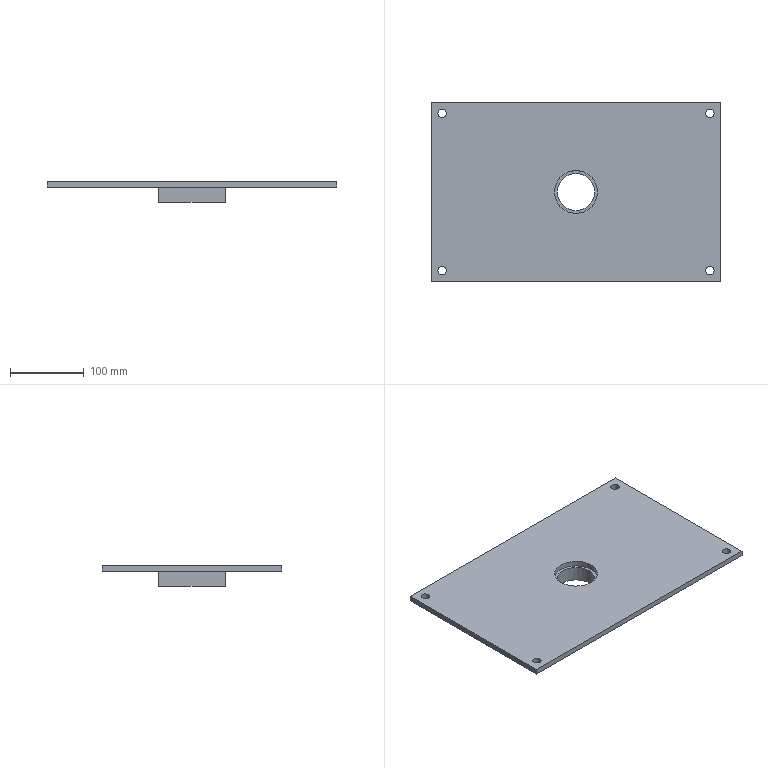Part | SolidWorks | features ICE 3, Extrusion 1, Scale 1 | 1 solid | 24 faces | box 393.75 x 243.75 x 28.125 mm | volume 822488 mm3 | cylinder 12 | plane 12 | commonest cylinder face diameters 11.25 x8 50.625 x2 58.125 x2
STEP:
#1=CARTESIAN_POINT('',(-29.062,0.,6.752));
#2=VERTEX_POINT('',#1);
#3=CARTESIAN_POINT('',(29.063,0.,6.752));
#4=VERTEX_POINT('',#3);
#5=CARTESIAN_POINT('',(0.,0.,6.752));
#6=DIRECTION('',(0.,0.,1.));
#7=DIRECTION('',(1.,0.,0.));
#8=AXIS2_PLACEMENT_3D('',#5,#6,#7);
#9=CIRCLE('',#8,29.062);
#10=EDGE_CURVE('',#2,#4,#9,.T.);
#11=ORIENTED_EDGE('',*,*,#10,.T.);
#12=CARTESIAN_POINT('',(29.063,0.,-0.7483));
#13=VERTEX_POINT('',#12);
#14=CARTESIAN_POINT('',(29.063,0.,19.877));
#15=DIRECTION('',(0.,0.,-1.));
#16=VECTOR('',#15,1000.);
#17=LINE('',#14,#16);
#18=EDGE_CURVE('',#4,#13,#17,.T.);
#19=ORIENTED_EDGE('',*,*,#18,.T.);
#20=CARTESIAN_POINT('',(-29.062,0.,-0.7483));
#21=VERTEX_POINT('',#20);
#22=CARTESIAN_POINT('',(0.,0.,-0.7483));
#23=DIRECTION('',(0.,0.,-1.));
#24=DIRECTION('',(-1.,0.,0.));
#25=AXIS2_PLACEMENT_3D('',#22,#23,#24);
#26=CIRCLE('',#25,29.062);
#27=EDGE_CURVE('',#13,#21,#26,.T.);
#28=ORIENTED_EDGE('',*,*,#27,.T.);
#29=CARTESIAN_POINT('',(-29.062,0.,19.877));
#30=DIRECTION('',(0.,0.,-1.));
#31=VECTOR('',#30,1000.);
#32=LINE('',#29,#31);
#33=EDGE_CURVE('',#2,#21,#32,.T.);
#34=ORIENTED_EDGE('',*,*,#33,.F.);
#35=EDGE_LOOP('',(#11,#19,#28,#34));
#36=FACE_OUTER_BOUND('',#35,.T.);
#37=CARTESIAN_POINT('',(0.,0.,19.877));
#38=DIRECTION('',(0.,0.,-1.));
#39=DIRECTION('',(-1.,0.,0.));
#40=AXIS2_PLACEMENT_3D('',#37,#38,#39);
#41=CYLINDRICAL_SURFACE('',#40,29.062);
#42=ADVANCED_FACE('',(#36),#41,.F.);
#43=CARTESIAN_POINT('',(-25.312,0.,-0.7483));
#44=VERTEX_POINT('',#43);
#45=CARTESIAN_POINT('',(25.313,0.,-0.7483));
#46=VERTEX_POINT('',#45);
#47=CARTESIAN_POINT('',(0.,0.,-0.7483));
#48=DIRECTION('',(0.,0.,1.));
#49=DIRECTION('',(-1.,0.,0.));
#50=AXIS2_PLACEMENT_3D('',#47,#48,#49);
#51=CIRCLE('',#50,25.312);
#52=EDGE_CURVE('',#44,#46,#51,.T.);
#53=ORIENTED_EDGE('',*,*,#52,.T.);
#54=CARTESIAN_POINT('',(25.313,0.,-21.373));
#55=VERTEX_POINT('',#54);
#56=CARTESIAN_POINT('',(25.313,0.,-0.7483));
#57=DIRECTION('',(0.,0.,-1.));
#58=VECTOR('',#57,1000.);
#59=LINE('',#56,#58);
#60=EDGE_CURVE('',#46,#55,#59,.T.);
#61=ORIENTED_EDGE('',*,*,#60,.T.);
#62=CARTESIAN_POINT('',(-25.312,0.,-21.373));
#63=VERTEX_POINT('',#62);
#64=CARTESIAN_POINT('',(0.,0.,-21.373));
#65=DIRECTION('',(0.,0.,-1.));
#66=DIRECTION('',(-1.,0.,0.));
#67=AXIS2_PLACEMENT_3D('',#64,#65,#66);
#68=CIRCLE('',#67,25.312);
#69=EDGE_CURVE('',#55,#63,#68,.T.);
#70=ORIENTED_EDGE('',*,*,#69,.T.);
#71=CARTESIAN_POINT('',(-25.312,0.,-0.7483));
#72=DIRECTION('',(0.,0.,-1.));
#73=VECTOR('',#72,1000.);
#74=LINE('',#71,#73);
#75=EDGE_CURVE('',#44,#63,#74,.T.);
#76=ORIENTED_EDGE('',*,*,#75,.F.);
#77=EDGE_LOOP('',(#53,#61,#70,#76));
#78=FACE_OUTER_BOUND('',#77,.T.);
#79=CARTESIAN_POINT('',(0.,0.,-0.7483));
#80=DIRECTION('',(0.,0.,-1.));
#81=DIRECTION('',(-1.,0.,0.));
#82=AXIS2_PLACEMENT_3D('',#79,#80,#81);
#83=CYLINDRICAL_SURFACE('',#82,25.312);
#84=ADVANCED_FACE('',(#78),#83,.F.);
#85=CARTESIAN_POINT('',(176.25,-106.875,6.752));
#86=VERTEX_POINT('',#85);
#87=CARTESIAN_POINT('',(187.5,-106.875,6.752));
#88=VERTEX_POINT('',#87);
#89=CARTESIAN_POINT('',(181.875,-106.875,6.752));
#90=DIRECTION('',(0.,0.,1.));
#91=DIRECTION('',(1.,0.,0.));
#92=AXIS2_PLACEMENT_3D('',#89,#90,#91);
#93=CIRCLE('',#92,5.625);
#94=EDGE_CURVE('',#86,#88,#93,.T.);
#95=ORIENTED_EDGE('',*,*,#94,.T.);
#96=CARTESIAN_POINT('',(187.5,-106.875,-0.7483));
#97=VERTEX_POINT('',#96);
#98=CARTESIAN_POINT('',(187.5,-106.875,6.752));
#99=DIRECTION('',(0.,0.,-1.));
#100=VECTOR('',#99,1000.);
#101=LINE('',#98,#100);
#102=EDGE_CURVE('',#88,#97,#101,.T.);
#103=ORIENTED_EDGE('',*,*,#102,.T.);
#104=CARTESIAN_POINT('',(176.25,-106.875,-0.7483));
#105=VERTEX_POINT('',#104);
#106=CARTESIAN_POINT('',(181.875,-106.875,-0.7483));
#107=DIRECTION('',(0.,0.,1.));
#108=DIRECTION('',(1.,0.,0.));
#109=AXIS2_PLACEMENT_3D('',#106,#107,#108);
#110=CIRCLE('',#109,5.625);
#111=EDGE_CURVE('',#105,#97,#110,.T.);
#112=ORIENTED_EDGE('',*,*,#111,.F.);
#113=CARTESIAN_POINT('',(176.25,-106.875,6.752));
#114=DIRECTION('',(0.,0.,-1.));
#115=VECTOR('',#114,1000.);
#116=LINE('',#113,#115);
#117=EDGE_CURVE('',#86,#105,#116,.T.);
#118=ORIENTED_EDGE('',*,*,#117,.F.);
#119=EDGE_LOOP('',(#95,#103,#112,#118));
#120=FACE_OUTER_BOUND('',#119,.T.);
#121=CARTESIAN_POINT('',(181.875,-106.875,6.752));
#122=DIRECTION('',(0.,0.,-1.));
#123=DIRECTION('',(-1.,0.,0.));
#124=AXIS2_PLACEMENT_3D('',#121,#122,#123);
#125=CYLINDRICAL_SURFACE('',#124,5.625);
#126=ADVANCED_FACE('',(#120),#125,.F.);
#127=CARTESIAN_POINT('',(-187.5,-106.875,6.752));
#128=VERTEX_POINT('',#127);
#129=CARTESIAN_POINT('',(-176.25,-106.875,6.752));
#130=VERTEX_POINT('',#129);
#131=CARTESIAN_POINT('',(-181.875,-106.875,6.752));
#132=DIRECTION('',(0.,0.,1.));
#133=DIRECTION('',(1.,0.,0.));
#134=AXIS2_PLACEMENT_3D('',#131,#132,#133);
#135=CIRCLE('',#134,5.625);
#136=EDGE_CURVE('',#128,#130,#135,.T.);
#137=ORIENTED_EDGE('',*,*,#136,.T.);
#138=CARTESIAN_POINT('',(-176.25,-106.875,-0.7483));
#139=VERTEX_POINT('',#138);
#140=CARTESIAN_POINT('',(-176.25,-106.875,6.752));
#141=DIRECTION('',(0.,0.,-1.));
#142=VECTOR('',#141,1000.);
#143=LINE('',#140,#142);
#144=EDGE_CURVE('',#130,#139,#143,.T.);
#145=ORIENTED_EDGE('',*,*,#144,.T.);
#146=CARTESIAN_POINT('',(-187.5,-106.875,-0.7483));
#147=VERTEX_POINT('',#146);
#148=CARTESIAN_POINT('',(-181.875,-106.875,-0.7483));
#149=DIRECTION('',(0.,0.,1.));
#150=DIRECTION('',(1.,0.,0.));
#151=AXIS2_PLACEMENT_3D('',#148,#149,#150);
#152=CIRCLE('',#151,5.625);
#153=EDGE_CURVE('',#147,#139,#152,.T.);
#154=ORIENTED_EDGE('',*,*,#153,.F.);
#155=CARTESIAN_POINT('',(-187.5,-106.875,6.752));
#156=DIRECTION('',(0.,0.,-1.));
#157=VECTOR('',#156,1000.);
#158=LINE('',#155,#157);
#159=EDGE_CURVE('',#128,#147,#158,.T.);
#160=ORIENTED_EDGE('',*,*,#159,.F.);
#161=EDGE_LOOP('',(#137,#145,#154,#160));
#162=FACE_OUTER_BOUND('',#161,.T.);
#163=CARTESIAN_POINT('',(-181.875,-106.875,6.752));
#164=DIRECTION('',(0.,0.,-1.));
#165=DIRECTION('',(-1.,0.,0.));
#166=AXIS2_PLACEMENT_3D('',#163,#164,#165);
#167=CYLINDRICAL_SURFACE('',#166,5.625);
#168=ADVANCED_FACE('',(#162),#167,.F.);
#169=CARTESIAN_POINT('',(-187.5,106.875,6.752));
#170=VERTEX_POINT('',#169);
#171=CARTESIAN_POINT('',(-176.25,106.875,6.752));
#172=VERTEX_POINT('',#171);
#173=CARTESIAN_POINT('',(-181.875,106.875,6.752));
#174=DIRECTION('',(0.,0.,1.));
#175=DIRECTION('',(1.,0.,0.));
#176=AXIS2_PLACEMENT_3D('',#173,#174,#175);
#177=CIRCLE('',#176,5.625);
#178=EDGE_CURVE('',#170,#172,#177,.T.);
#179=ORIENTED_EDGE('',*,*,#178,.T.);
#180=CARTESIAN_POINT('',(-176.25,106.875,-0.7483));
#181=VERTEX_POINT('',#180);
#182=CARTESIAN_POINT('',(-176.25,106.875,6.752));
#183=DIRECTION('',(0.,0.,-1.));
#184=VECTOR('',#183,1000.);
#185=LINE('',#182,#184);
#186=EDGE_CURVE('',#172,#181,#185,.T.);
#187=ORIENTED_EDGE('',*,*,#186,.T.);
#188=CARTESIAN_POINT('',(-187.5,106.875,-0.7483));
#189=VERTEX_POINT('',#188);
#190=CARTESIAN_POINT('',(-181.875,106.875,-0.7483));
#191=DIRECTION('',(0.,0.,1.));
#192=DIRECTION('',(1.,0.,0.));
#193=AXIS2_PLACEMENT_3D('',#190,#191,#192);
#194=CIRCLE('',#193,5.625);
#195=EDGE_CURVE('',#189,#181,#194,.T.);
#196=ORIENTED_EDGE('',*,*,#195,.F.);
#197=CARTESIAN_POINT('',(-187.5,106.875,6.752));
#198=DIRECTION('',(0.,0.,-1.));
#199=VECTOR('',#198,1000.);
#200=LINE('',#197,#199);
#201=EDGE_CURVE('',#170,#189,#200,.T.);
#202=ORIENTED_EDGE('',*,*,#201,.F.);
#203=EDGE_LOOP('',(#179,#187,#196,#202));
#204=FACE_OUTER_BOUND('',#203,.T.);
#205=CARTESIAN_POINT('',(-181.875,106.875,6.752));
#206=DIRECTION('',(0.,0.,-1.));
#207=DIRECTION('',(-1.,0.,0.));
#208=AXIS2_PLACEMENT_3D('',#205,#206,#207);
#209=CYLINDRICAL_SURFACE('',#208,5.625);
#210=ADVANCED_FACE('',(#204),#209,.F.);
#211=CARTESIAN_POINT('',(176.25,106.875,6.752));
#212=VERTEX_POINT('',#211);
#213=CARTESIAN_POINT('',(187.5,106.875,6.752));
#214=VERTEX_POINT('',#213);
#215=CARTESIAN_POINT('',(181.875,106.875,6.752));
#216=DIRECTION('',(0.,0.,1.));
#217=DIRECTION('',(1.,0.,0.));
#218=AXIS2_PLACEMENT_3D('',#215,#216,#217);
#219=CIRCLE('',#218,5.625);
#220=EDGE_CURVE('',#212,#214,#219,.T.);
#221=ORIENTED_EDGE('',*,*,#220,.T.);
#222=CARTESIAN_POINT('',(187.5,106.875,-0.7483));
#223=VERTEX_POINT('',#222);
#224=CARTESIAN_POINT('',(187.5,106.875,6.752));
#225=DIRECTION('',(0.,0.,-1.));
#226=VECTOR('',#225,1000.);
#227=LINE('',#224,#226);
#228=EDGE_CURVE('',#214,#223,#227,.T.);
#229=ORIENTED_EDGE('',*,*,#228,.T.);
#230=CARTESIAN_POINT('',(176.25,106.875,-0.7483));
#231=VERTEX_POINT('',#230);
#232=CARTESIAN_POINT('',(181.875,106.875,-0.7483));
#233=DIRECTION('',(0.,0.,1.));
#234=DIRECTION('',(1.,0.,0.));
#235=AXIS2_PLACEMENT_3D('',#232,#233,#234);
#236=CIRCLE('',#235,5.625);
#237=EDGE_CURVE('',#231,#223,#236,.T.);
#238=ORIENTED_EDGE('',*,*,#237,.F.);
#239=CARTESIAN_POINT('',(176.25,106.875,6.752));
#240=DIRECTION('',(0.,0.,-1.));
#241=VECTOR('',#240,1000.);
#242=LINE('',#239,#241);
#243=EDGE_CURVE('',#212,#231,#242,.T.);
#244=ORIENTED_EDGE('',*,*,#243,.F.);
#245=EDGE_LOOP('',(#221,#229,#238,#244));
#246=FACE_OUTER_BOUND('',#245,.T.);
#247=CARTESIAN_POINT('',(181.875,106.875,6.752));
#248=DIRECTION('',(0.,0.,-1.));
#249=DIRECTION('',(-1.,0.,0.));
#250=AXIS2_PLACEMENT_3D('',#247,#248,#249);
#251=CYLINDRICAL_SURFACE('',#250,5.625);
#252=ADVANCED_FACE('',(#246),#251,.F.);
#253=ORIENTED_EDGE('',*,*,#111,.T.);
#254=CARTESIAN_POINT('',(181.875,-106.875,-0.7483));
#255=DIRECTION('',(0.,0.,1.));
#256=DIRECTION('',(1.,0.,0.));
#257=AXIS2_PLACEMENT_3D('',#254,#255,#256);
#258=CIRCLE('',#257,5.625);
#259=EDGE_CURVE('',#97,#105,#258,.T.);
#260=ORIENTED_EDGE('',*,*,#259,.T.);
#261=EDGE_LOOP('',(#253,#260));
#262=FACE_BOUND('',#261,.T.);
#263=ORIENTED_EDGE('',*,*,#195,.T.);
#264=CARTESIAN_POINT('',(-181.875,106.875,-0.7483));
#265=DIRECTION('',(0.,0.,1.));
#266=DIRECTION('',(1.,0.,0.));
#267=AXIS2_PLACEMENT_3D('',#264,#265,#266);
#268=CIRCLE('',#267,5.625);
#269=EDGE_CURVE('',#181,#189,#268,.T.);
#270=ORIENTED_EDGE('',*,*,#269,.T.);
#271=EDGE_LOOP('',(#263,#270));
#272=FACE_BOUND('',#271,.T.);
#273=CARTESIAN_POINT('',(-196.875,121.875,-0.7483));
#274=VERTEX_POINT('',#273);
#275=CARTESIAN_POINT('',(-196.875,-121.875,-0.7483));
#276=VERTEX_POINT('',#275);
#277=CARTESIAN_POINT('',(-196.875,121.875,-0.7483));
#278=DIRECTION('',(0.,-1.,0.));
#279=VECTOR('',#278,1000.);
#280=LINE('',#277,#279);
#281=EDGE_CURVE('',#274,#276,#280,.T.);
#282=ORIENTED_EDGE('',*,*,#281,.F.);
#283=CARTESIAN_POINT('',(196.875,121.875,-0.7483));
#284=VERTEX_POINT('',#283);
#285=CARTESIAN_POINT('',(-196.875,121.875,-0.7483));
#286=DIRECTION('',(-1.,0.,0.));
#287=VECTOR('',#286,1000.);
#288=LINE('',#285,#287);
#289=EDGE_CURVE('',#284,#274,#288,.T.);
#290=ORIENTED_EDGE('',*,*,#289,.F.);
#291=CARTESIAN_POINT('',(196.875,-121.875,-0.7483));
#292=VERTEX_POINT('',#291);
#293=CARTESIAN_POINT('',(196.875,121.875,-0.7483));
#294=DIRECTION('',(0.,1.,0.));
#295=VECTOR('',#294,1000.);
#296=LINE('',#293,#295);
#297=EDGE_CURVE('',#292,#284,#296,.T.);
#298=ORIENTED_EDGE('',*,*,#297,.F.);
#299=CARTESIAN_POINT('',(-196.875,-121.875,-0.7483));
#300=DIRECTION('',(1.,0.,0.));
#301=VECTOR('',#300,1000.);
#302=LINE('',#299,#301);
#303=EDGE_CURVE('',#276,#292,#302,.T.);
#304=ORIENTED_EDGE('',*,*,#303,.F.);
#305=EDGE_LOOP('',(#282,#290,#298,#304));
#306=FACE_OUTER_BOUND('',#305,.T.);
#307=ORIENTED_EDGE('',*,*,#237,.T.);
#308=CARTESIAN_POINT('',(181.875,106.875,-0.7483));
#309=DIRECTION('',(0.,0.,1.));
#310=DIRECTION('',(1.,0.,0.));
#311=AXIS2_PLACEMENT_3D('',#308,#309,#310);
#312=CIRCLE('',#311,5.625);
#313=EDGE_CURVE('',#223,#231,#312,.T.);
#314=ORIENTED_EDGE('',*,*,#313,.T.);
#315=EDGE_LOOP('',(#307,#314));
#316=FACE_BOUND('',#315,.T.);
#317=ORIENTED_EDGE('',*,*,#153,.T.);
#318=CARTESIAN_POINT('',(-181.875,-106.875,-0.7483));
#319=DIRECTION('',(0.,0.,1.));
#320=DIRECTION('',(1.,0.,0.));
#321=AXIS2_PLACEMENT_3D('',#318,#319,#320);
#322=CIRCLE('',#321,5.625);
#323=EDGE_CURVE('',#139,#147,#322,.T.);
#324=ORIENTED_EDGE('',*,*,#323,.T.);
#325=EDGE_LOOP('',(#317,#324));
#326=FACE_BOUND('',#325,.T.);
#327=CARTESIAN_POINT('',(45.,45.,-0.7483));
#328=VERTEX_POINT('',#327);
#329=CARTESIAN_POINT('',(45.,-45.,-0.7483));
#330=VERTEX_POINT('',#329);
#331=CARTESIAN_POINT('',(45.,45.,-0.7483));
#332=DIRECTION('',(0.,-1.,0.));
#333=VECTOR('',#332,1000.);
#334=LINE('',#331,#333);
#335=EDGE_CURVE('',#328,#330,#334,.T.);
#336=ORIENTED_EDGE('',*,*,#335,.F.);
#337=CARTESIAN_POINT('',(-45.,45.,-0.7483));
#338=VERTEX_POINT('',#337);
#339=CARTESIAN_POINT('',(45.,45.,-0.7483));
#340=DIRECTION('',(1.,0.,0.));
#341=VECTOR('',#340,1000.);
#342=LINE('',#339,#341);
#343=EDGE_CURVE('',#338,#328,#342,.T.);
#344=ORIENTED_EDGE('',*,*,#343,.F.);
#345=CARTESIAN_POINT('',(-45.,-45.,-0.7483));
#346=VERTEX_POINT('',#345);
#347=CARTESIAN_POINT('',(-45.,45.,-0.7483));
#348=DIRECTION('',(0.,1.,0.));
#349=VECTOR('',#348,1000.);
#350=LINE('',#347,#349);
#351=EDGE_CURVE('',#346,#338,#350,.T.);
#352=ORIENTED_EDGE('',*,*,#351,.F.);
#353=CARTESIAN_POINT('',(45.,-45.,-0.7483));
#354=DIRECTION('',(-1.,0.,0.));
#355=VECTOR('',#354,1000.);
#356=LINE('',#353,#355);
#357=EDGE_CURVE('',#330,#346,#356,.T.);
#358=ORIENTED_EDGE('',*,*,#357,.F.);
#359=EDGE_LOOP('',(#336,#344,#352,#358));
#360=FACE_BOUND('',#359,.T.);
#361=CARTESIAN_POINT('',(0.,0.,-0.7483));
#362=DIRECTION('',(0.,0.,1.));
#363=DIRECTION('',(1.,0.,0.));
#364=AXIS2_PLACEMENT_3D('',#361,#362,#363);
#365=PLANE('',#364);
#366=ADVANCED_FACE('',(#262,#272,#306,#316,#326,#360),#365,.F.);
#367=ORIENTED_EDGE('',*,*,#10,.F.);
#368=CARTESIAN_POINT('',(0.,0.,6.752));
#369=DIRECTION('',(0.,0.,1.));
#370=DIRECTION('',(1.,0.,0.));
#371=AXIS2_PLACEMENT_3D('',#368,#369,#370);
#372=CIRCLE('',#371,29.062);
#373=EDGE_CURVE('',#4,#2,#372,.T.);
#374=ORIENTED_EDGE('',*,*,#373,.F.);
#375=EDGE_LOOP('',(#367,#374));
#376=FACE_BOUND('',#375,.T.);
#377=ORIENTED_EDGE('',*,*,#136,.F.);
#378=CARTESIAN_POINT('',(-181.875,-106.875,6.752));
#379=DIRECTION('',(0.,0.,1.));
#380=DIRECTION('',(1.,0.,0.));
#381=AXIS2_PLACEMENT_3D('',#378,#379,#380);
#382=CIRCLE('',#381,5.625);
#383=EDGE_CURVE('',#130,#128,#382,.T.);
#384=ORIENTED_EDGE('',*,*,#383,.F.);
#385=EDGE_LOOP('',(#377,#384));
#386=FACE_BOUND('',#385,.T.);
#387=ORIENTED_EDGE('',*,*,#220,.F.);
#388=CARTESIAN_POINT('',(181.875,106.875,6.752));
#389=DIRECTION('',(0.,0.,1.));
#390=DIRECTION('',(1.,0.,0.));
#391=AXIS2_PLACEMENT_3D('',#388,#389,#390);
#392=CIRCLE('',#391,5.625);
#393=EDGE_CURVE('',#214,#212,#392,.T.);
#394=ORIENTED_EDGE('',*,*,#393,.F.);
#395=EDGE_LOOP('',(#387,#394));
#396=FACE_BOUND('',#395,.T.);
#397=CARTESIAN_POINT('',(-196.875,121.875,6.752));
#398=VERTEX_POINT('',#397);
#399=CARTESIAN_POINT('',(-196.875,-121.875,6.752));
#400=VERTEX_POINT('',#399);
#401=CARTESIAN_POINT('',(-196.875,121.875,6.752));
#402=DIRECTION('',(0.,-1.,0.));
#403=VECTOR('',#402,1000.);
#404=LINE('',#401,#403);
#405=EDGE_CURVE('',#398,#400,#404,.T.);
#406=ORIENTED_EDGE('',*,*,#405,.T.);
#407=CARTESIAN_POINT('',(196.875,-121.875,6.752));
#408=VERTEX_POINT('',#407);
#409=CARTESIAN_POINT('',(-196.875,-121.875,6.752));
#410=DIRECTION('',(1.,0.,0.));
#411=VECTOR('',#410,1000.);
#412=LINE('',#409,#411);
#413=EDGE_CURVE('',#400,#408,#412,.T.);
#414=ORIENTED_EDGE('',*,*,#413,.T.);
#415=CARTESIAN_POINT('',(196.875,121.875,6.752));
#416=VERTEX_POINT('',#415);
#417=CARTESIAN_POINT('',(196.875,121.875,6.752));
#418=DIRECTION('',(0.,1.,0.));
#419=VECTOR('',#418,1000.);
#420=LINE('',#417,#419);
#421=EDGE_CURVE('',#408,#416,#420,.T.);
#422=ORIENTED_EDGE('',*,*,#421,.T.);
#423=CARTESIAN_POINT('',(-196.875,121.875,6.752));
#424=DIRECTION('',(-1.,0.,0.));
#425=VECTOR('',#424,1000.);
#426=LINE('',#423,#425);
#427=EDGE_CURVE('',#416,#398,#426,.T.);
#428=ORIENTED_EDGE('',*,*,#427,.T.);
#429=EDGE_LOOP('',(#406,#414,#422,#428));
#430=FACE_OUTER_BOUND('',#429,.T.);
#431=ORIENTED_EDGE('',*,*,#178,.F.);
#432=CARTESIAN_POINT('',(-181.875,106.875,6.752));
#433=DIRECTION('',(0.,0.,1.));
#434=DIRECTION('',(1.,0.,0.));
#435=AXIS2_PLACEMENT_3D('',#432,#433,#434);
#436=CIRCLE('',#435,5.625);
#437=EDGE_CURVE('',#172,#170,#436,.T.);
#438=ORIENTED_EDGE('',*,*,#437,.F.);
#439=EDGE_LOOP('',(#431,#438));
#440=FACE_BOUND('',#439,.T.);
#441=ORIENTED_EDGE('',*,*,#94,.F.);
#442=CARTESIAN_POINT('',(181.875,-106.875,6.752));
#443=DIRECTION('',(0.,0.,1.));
#444=DIRECTION('',(1.,0.,0.));
#445=AXIS2_PLACEMENT_3D('',#442,#443,#444);
#446=CIRCLE('',#445,5.625);
#447=EDGE_CURVE('',#88,#86,#446,.T.);
#448=ORIENTED_EDGE('',*,*,#447,.F.);
#449=EDGE_LOOP('',(#441,#448));
#450=FACE_BOUND('',#449,.T.);
#451=CARTESIAN_POINT('',(0.,0.,6.752));
#452=DIRECTION('',(0.,0.,1.));
#453=DIRECTION('',(1.,0.,0.));
#454=AXIS2_PLACEMENT_3D('',#451,#452,#453);
#455=PLANE('',#454);
#456=ADVANCED_FACE('',(#376,#386,#396,#430,#440,#450),#455,.T.);
#457=ORIENTED_EDGE('',*,*,#281,.T.);
#458=CARTESIAN_POINT('',(-196.875,-121.875,6.752));
#459=DIRECTION('',(0.,0.,-1.));
#460=VECTOR('',#459,1000.);
#461=LINE('',#458,#460);
#462=EDGE_CURVE('',#400,#276,#461,.T.);
#463=ORIENTED_EDGE('',*,*,#462,.F.);
#464=ORIENTED_EDGE('',*,*,#405,.F.);
#465=CARTESIAN_POINT('',(-196.875,121.875,6.752));
#466=DIRECTION('',(0.,0.,-1.));
#467=VECTOR('',#466,1000.);
#468=LINE('',#465,#467);
#469=EDGE_CURVE('',#398,#274,#468,.T.);
#470=ORIENTED_EDGE('',*,*,#469,.T.);
#471=EDGE_LOOP('',(#457,#463,#464,#470));
#472=FACE_OUTER_BOUND('',#471,.T.);
#473=CARTESIAN_POINT('',(-196.875,121.875,6.752));
#474=DIRECTION('',(1.,0.,0.));
#475=DIRECTION('',(0.,0.,-1.));
#476=AXIS2_PLACEMENT_3D('',#473,#474,#475);
#477=PLANE('',#476);
#478=ADVANCED_FACE('',(#472),#477,.F.);
#479=ORIENTED_EDGE('',*,*,#303,.T.);
#480=CARTESIAN_POINT('',(196.875,-121.875,6.752));
#481=DIRECTION('',(0.,0.,-1.));
#482=VECTOR('',#481,1000.);
#483=LINE('',#480,#482);
#484=EDGE_CURVE('',#408,#292,#483,.T.);
#485=ORIENTED_EDGE('',*,*,#484,.F.);
#486=ORIENTED_EDGE('',*,*,#413,.F.);
#487=ORIENTED_EDGE('',*,*,#462,.T.);
#488=EDGE_LOOP('',(#479,#485,#486,#487));
#489=FACE_OUTER_BOUND('',#488,.T.);
#490=CARTESIAN_POINT('',(-196.875,-121.875,6.752));
#491=DIRECTION('',(0.,1.,0.));
#492=DIRECTION('',(-1.,0.,0.));
#493=AXIS2_PLACEMENT_3D('',#490,#491,#492);
#494=PLANE('',#493);
#495=ADVANCED_FACE('',(#489),#494,.F.);
#496=ORIENTED_EDGE('',*,*,#297,.T.);
#497=CARTESIAN_POINT('',(196.875,121.875,6.752));
#498=DIRECTION('',(0.,0.,-1.));
#499=VECTOR('',#498,1000.);
#500=LINE('',#497,#499);
#501=EDGE_CURVE('',#416,#284,#500,.T.);
#502=ORIENTED_EDGE('',*,*,#501,.F.);
#503=ORIENTED_EDGE('',*,*,#421,.F.);
#504=ORIENTED_EDGE('',*,*,#484,.T.);
#505=EDGE_LOOP('',(#496,#502,#503,#504));
#506=FACE_OUTER_BOUND('',#505,.T.);
#507=CARTESIAN_POINT('',(196.875,121.875,6.752));
#508=DIRECTION('',(-1.,0.,0.));
#509=DIRECTION('',(0.,0.,1.));
#510=AXIS2_PLACEMENT_3D('',#507,#508,#509);
#511=PLANE('',#510);
#512=ADVANCED_FACE('',(#506),#511,.F.);
#513=ORIENTED_EDGE('',*,*,#289,.T.);
#514=ORIENTED_EDGE('',*,*,#469,.F.);
#515=ORIENTED_EDGE('',*,*,#427,.F.);
#516=ORIENTED_EDGE('',*,*,#501,.T.);
#517=EDGE_LOOP('',(#513,#514,#515,#516));
#518=FACE_OUTER_BOUND('',#517,.T.);
#519=CARTESIAN_POINT('',(-196.875,121.875,6.752));
#520=DIRECTION('',(0.,-1.,0.));
#521=DIRECTION('',(0.,0.,-1.));
#522=AXIS2_PLACEMENT_3D('',#519,#520,#521);
#523=PLANE('',#522);
#524=ADVANCED_FACE('',(#518),#523,.F.);
#525=ORIENTED_EDGE('',*,*,#228,.F.);
#526=ORIENTED_EDGE('',*,*,#393,.T.);
#527=ORIENTED_EDGE('',*,*,#243,.T.);
#528=ORIENTED_EDGE('',*,*,#313,.F.);
#529=EDGE_LOOP('',(#525,#526,#527,#528));
#530=FACE_OUTER_BOUND('',#529,.T.);
#531=CARTESIAN_POINT('',(181.875,106.875,6.752));
#532=DIRECTION('',(0.,0.,-1.));
#533=DIRECTION('',(-1.,0.,0.));
#534=AXIS2_PLACEMENT_3D('',#531,#532,#533);
#535=CYLINDRICAL_SURFACE('',#534,5.625);
#536=ADVANCED_FACE('',(#530),#535,.F.);
#537=ORIENTED_EDGE('',*,*,#186,.F.);
#538=ORIENTED_EDGE('',*,*,#437,.T.);
#539=ORIENTED_EDGE('',*,*,#201,.T.);
#540=ORIENTED_EDGE('',*,*,#269,.F.);
#541=EDGE_LOOP('',(#537,#538,#539,#540));
#542=FACE_OUTER_BOUND('',#541,.T.);
#543=CARTESIAN_POINT('',(-181.875,106.875,6.752));
#544=DIRECTION('',(0.,0.,-1.));
#545=DIRECTION('',(-1.,0.,0.));
#546=AXIS2_PLACEMENT_3D('',#543,#544,#545);
#547=CYLINDRICAL_SURFACE('',#546,5.625);
#548=ADVANCED_FACE('',(#542),#547,.F.);
#549=ORIENTED_EDGE('',*,*,#144,.F.);
#550=ORIENTED_EDGE('',*,*,#383,.T.);
#551=ORIENTED_EDGE('',*,*,#159,.T.);
#552=ORIENTED_EDGE('',*,*,#323,.F.);
#553=EDGE_LOOP('',(#549,#550,#551,#552));
#554=FACE_OUTER_BOUND('',#553,.T.);
#555=CARTESIAN_POINT('',(-181.875,-106.875,6.752));
#556=DIRECTION('',(0.,0.,-1.));
#557=DIRECTION('',(-1.,0.,0.));
#558=AXIS2_PLACEMENT_3D('',#555,#556,#557);
#559=CYLINDRICAL_SURFACE('',#558,5.625);
#560=ADVANCED_FACE('',(#554),#559,.F.);
#561=ORIENTED_EDGE('',*,*,#102,.F.);
#562=ORIENTED_EDGE('',*,*,#447,.T.);
#563=ORIENTED_EDGE('',*,*,#117,.T.);
#564=ORIENTED_EDGE('',*,*,#259,.F.);
#565=EDGE_LOOP('',(#561,#562,#563,#564));
#566=FACE_OUTER_BOUND('',#565,.T.);
#567=CARTESIAN_POINT('',(181.875,-106.875,6.752));
#568=DIRECTION('',(0.,0.,-1.));
#569=DIRECTION('',(-1.,0.,0.));
#570=AXIS2_PLACEMENT_3D('',#567,#568,#569);
#571=CYLINDRICAL_SURFACE('',#570,5.625);
#572=ADVANCED_FACE('',(#566),#571,.F.);
#573=ORIENTED_EDGE('',*,*,#335,.T.);
#574=CARTESIAN_POINT('',(45.,-45.,-21.373));
#575=VERTEX_POINT('',#574);
#576=CARTESIAN_POINT('',(45.,-45.,-21.373));
#577=DIRECTION('',(0.,0.,1.));
#578=VECTOR('',#577,1000.);
#579=LINE('',#576,#578);
#580=EDGE_CURVE('',#575,#330,#579,.T.);
#581=ORIENTED_EDGE('',*,*,#580,.F.);
#582=CARTESIAN_POINT('',(45.,45.,-21.373));
#583=VERTEX_POINT('',#582);
#584=CARTESIAN_POINT('',(45.,45.,-21.373));
#585=DIRECTION('',(0.,-1.,0.));
#586=VECTOR('',#585,1000.);
#587=LINE('',#584,#586);
#588=EDGE_CURVE('',#583,#575,#587,.T.);
#589=ORIENTED_EDGE('',*,*,#588,.F.);
#590=CARTESIAN_POINT('',(45.,45.,-21.373));
#591=DIRECTION('',(0.,0.,1.));
#592=VECTOR('',#591,1000.);
#593=LINE('',#590,#592);
#594=EDGE_CURVE('',#583,#328,#593,.T.);
#595=ORIENTED_EDGE('',*,*,#594,.T.);
#596=EDGE_LOOP('',(#573,#581,#589,#595));
#597=FACE_OUTER_BOUND('',#596,.T.);
#598=CARTESIAN_POINT('',(45.,45.,-21.373));
#599=DIRECTION('',(-1.,0.,0.));
#600=DIRECTION('',(0.,-1.,0.));
#601=AXIS2_PLACEMENT_3D('',#598,#599,#600);
#602=PLANE('',#601);
#603=ADVANCED_FACE('',(#597),#602,.F.);
#604=ORIENTED_EDGE('',*,*,#357,.T.);
#605=CARTESIAN_POINT('',(-45.,-45.,-21.373));
#606=VERTEX_POINT('',#605);
#607=CARTESIAN_POINT('',(-45.,-45.,-21.373));
#608=DIRECTION('',(0.,0.,1.));
#609=VECTOR('',#608,1000.);
#610=LINE('',#607,#609);
#611=EDGE_CURVE('',#606,#346,#610,.T.);
#612=ORIENTED_EDGE('',*,*,#611,.F.);
#613=CARTESIAN_POINT('',(45.,-45.,-21.373));
#614=DIRECTION('',(-1.,0.,0.));
#615=VECTOR('',#614,1000.);
#616=LINE('',#613,#615);
#617=EDGE_CURVE('',#575,#606,#616,.T.);
#618=ORIENTED_EDGE('',*,*,#617,.F.);
#619=ORIENTED_EDGE('',*,*,#580,.T.);
#620=EDGE_LOOP('',(#604,#612,#618,#619));
#621=FACE_OUTER_BOUND('',#620,.T.);
#622=CARTESIAN_POINT('',(45.,-45.,-21.373));
#623=DIRECTION('',(0.,1.,0.));
#624=DIRECTION('',(-1.,0.,0.));
#625=AXIS2_PLACEMENT_3D('',#622,#623,#624);
#626=PLANE('',#625);
#627=ADVANCED_FACE('',(#621),#626,.F.);
#628=ORIENTED_EDGE('',*,*,#351,.T.);
#629=CARTESIAN_POINT('',(-45.,45.,-21.373));
#630=VERTEX_POINT('',#629);
#631=CARTESIAN_POINT('',(-45.,45.,-21.373));
#632=DIRECTION('',(0.,0.,1.));
#633=VECTOR('',#632,1000.);
#634=LINE('',#631,#633);
#635=EDGE_CURVE('',#630,#338,#634,.T.);
#636=ORIENTED_EDGE('',*,*,#635,.F.);
#637=CARTESIAN_POINT('',(-45.,45.,-21.373));
#638=DIRECTION('',(0.,1.,0.));
#639=VECTOR('',#638,1000.);
#640=LINE('',#637,#639);
#641=EDGE_CURVE('',#606,#630,#640,.T.);
#642=ORIENTED_EDGE('',*,*,#641,.F.);
#643=ORIENTED_EDGE('',*,*,#611,.T.);
#644=EDGE_LOOP('',(#628,#636,#642,#643));
#645=FACE_OUTER_BOUND('',#644,.T.);
#646=CARTESIAN_POINT('',(-45.,45.,-21.373));
#647=DIRECTION('',(1.,0.,0.));
#648=DIRECTION('',(0.,1.,0.));
#649=AXIS2_PLACEMENT_3D('',#646,#647,#648);
#650=PLANE('',#649);
#651=ADVANCED_FACE('',(#645),#650,.F.);
#652=ORIENTED_EDGE('',*,*,#343,.T.);
#653=ORIENTED_EDGE('',*,*,#594,.F.);
#654=CARTESIAN_POINT('',(45.,45.,-21.373));
#655=DIRECTION('',(1.,0.,0.));
#656=VECTOR('',#655,1000.);
#657=LINE('',#654,#656);
#658=EDGE_CURVE('',#630,#583,#657,.T.);
#659=ORIENTED_EDGE('',*,*,#658,.F.);
#660=ORIENTED_EDGE('',*,*,#635,.T.);
#661=EDGE_LOOP('',(#652,#653,#659,#660));
#662=FACE_OUTER_BOUND('',#661,.T.);
#663=CARTESIAN_POINT('',(45.,45.,-21.373));
#664=DIRECTION('',(0.,-1.,0.));
#665=DIRECTION('',(0.,0.,-1.));
#666=AXIS2_PLACEMENT_3D('',#663,#664,#665);
#667=PLANE('',#666);
#668=ADVANCED_FACE('',(#662),#667,.F.);
#669=CARTESIAN_POINT('',(0.,0.,-21.373));
#670=DIRECTION('',(0.,0.,-1.));
#671=DIRECTION('',(-1.,0.,0.));
#672=AXIS2_PLACEMENT_3D('',#669,#670,#671);
#673=CIRCLE('',#672,25.312);
#674=EDGE_CURVE('',#63,#55,#673,.T.);
#675=ORIENTED_EDGE('',*,*,#674,.F.);
#676=ORIENTED_EDGE('',*,*,#69,.F.);
#677=EDGE_LOOP('',(#675,#676));
#678=FACE_BOUND('',#677,.T.);
#679=ORIENTED_EDGE('',*,*,#588,.T.);
#680=ORIENTED_EDGE('',*,*,#617,.T.);
#681=ORIENTED_EDGE('',*,*,#641,.T.);
#682=ORIENTED_EDGE('',*,*,#658,.T.);
#683=EDGE_LOOP('',(#679,#680,#681,#682));
#684=FACE_OUTER_BOUND('',#683,.T.);
#685=CARTESIAN_POINT('',(0.,0.,-21.373));
#686=DIRECTION('',(0.,0.,-1.));
#687=DIRECTION('',(-1.,0.,0.));
#688=AXIS2_PLACEMENT_3D('',#685,#686,#687);
#689=PLANE('',#688);
#690=ADVANCED_FACE('',(#678,#684),#689,.T.);
#691=ORIENTED_EDGE('',*,*,#60,.F.);
#692=CARTESIAN_POINT('',(0.,0.,-0.7483));
#693=DIRECTION('',(0.,0.,1.));
#694=DIRECTION('',(-1.,0.,0.));
#695=AXIS2_PLACEMENT_3D('',#692,#693,#694);
#696=CIRCLE('',#695,25.312);
#697=EDGE_CURVE('',#46,#44,#696,.T.);
#698=ORIENTED_EDGE('',*,*,#697,.T.);
#699=ORIENTED_EDGE('',*,*,#75,.T.);
#700=ORIENTED_EDGE('',*,*,#674,.T.);
#701=EDGE_LOOP('',(#691,#698,#699,#700));
#702=FACE_OUTER_BOUND('',#701,.T.);
#703=CARTESIAN_POINT('',(0.,0.,-0.7483));
#704=DIRECTION('',(0.,0.,-1.));
#705=DIRECTION('',(-1.,0.,0.));
#706=AXIS2_PLACEMENT_3D('',#703,#704,#705);
#707=CYLINDRICAL_SURFACE('',#706,25.312);
#708=ADVANCED_FACE('',(#702),#707,.F.);
#709=CARTESIAN_POINT('',(0.,0.,-0.7483));
#710=DIRECTION('',(0.,0.,-1.));
#711=DIRECTION('',(-1.,0.,0.));
#712=AXIS2_PLACEMENT_3D('',#709,#710,#711);
#713=CIRCLE('',#712,29.062);
#714=EDGE_CURVE('',#21,#13,#713,.T.);
#715=ORIENTED_EDGE('',*,*,#714,.F.);
#716=ORIENTED_EDGE('',*,*,#27,.F.);
#717=EDGE_LOOP('',(#715,#716));
#718=FACE_OUTER_BOUND('',#717,.T.);
#719=ORIENTED_EDGE('',*,*,#52,.F.);
#720=ORIENTED_EDGE('',*,*,#697,.F.);
#721=EDGE_LOOP('',(#719,#720));
#722=FACE_BOUND('',#721,.T.);
#723=CARTESIAN_POINT('',(0.,0.,-0.7483));
#724=DIRECTION('',(0.,0.,-1.));
#725=DIRECTION('',(-1.,0.,0.));
#726=AXIS2_PLACEMENT_3D('',#723,#724,#725);
#727=PLANE('',#726);
#728=ADVANCED_FACE('',(#718,#722),#727,.F.);
#729=ORIENTED_EDGE('',*,*,#18,.F.);
#730=ORIENTED_EDGE('',*,*,#373,.T.);
#731=ORIENTED_EDGE('',*,*,#33,.T.);
#732=ORIENTED_EDGE('',*,*,#714,.T.);
#733=EDGE_LOOP('',(#729,#730,#731,#732));
#734=FACE_OUTER_BOUND('',#733,.T.);
#735=CARTESIAN_POINT('',(0.,0.,19.877));
#736=DIRECTION('',(0.,0.,-1.));
#737=DIRECTION('',(-1.,0.,0.));
#738=AXIS2_PLACEMENT_3D('',#735,#736,#737);
#739=CYLINDRICAL_SURFACE('',#738,29.062);
#740=ADVANCED_FACE('',(#734),#739,.F.);
#741=CLOSED_SHELL('',(#42,#84,#126,#168,#210,#252,#366,#456,#478,#495,#512,#524,#536,#548,#560,#572,#603,#627,#651,#668,#690,#708,#728,#740));
#742=MANIFOLD_SOLID_BREP('',#741);
#743=CARTESIAN_POINT('',(0.,0.,0.));
#744=DIRECTION('',(0.,0.,1.));
#745=DIRECTION('',(1.,0.,0.));
#746=AXIS2_PLACEMENT_3D('',#743,#744,#745);
#747=(LENGTH_UNIT()NAMED_UNIT(*)SI_UNIT(.MILLI.,.METRE.));
#748=UNCERTAINTY_MEASURE_WITH_UNIT(LENGTH_MEASURE(0.00001),#747,'','');
#749=(NAMED_UNIT(*)PLANE_ANGLE_UNIT()SI_UNIT($,.RADIAN.));
#750=(NAMED_UNIT(*)SI_UNIT($,.STERADIAN.)SOLID_ANGLE_UNIT());
#751=(GEOMETRIC_REPRESENTATION_CONTEXT(3)GLOBAL_UNCERTAINTY_ASSIGNED_CONTEXT((#748))GLOBAL_UNIT_ASSIGNED_CONTEXT((#747,#749,#750))REPRESENTATION_CONTEXT('',''));
#752=ADVANCED_BREP_SHAPE_REPRESENTATION('',(#742,#746),#751);